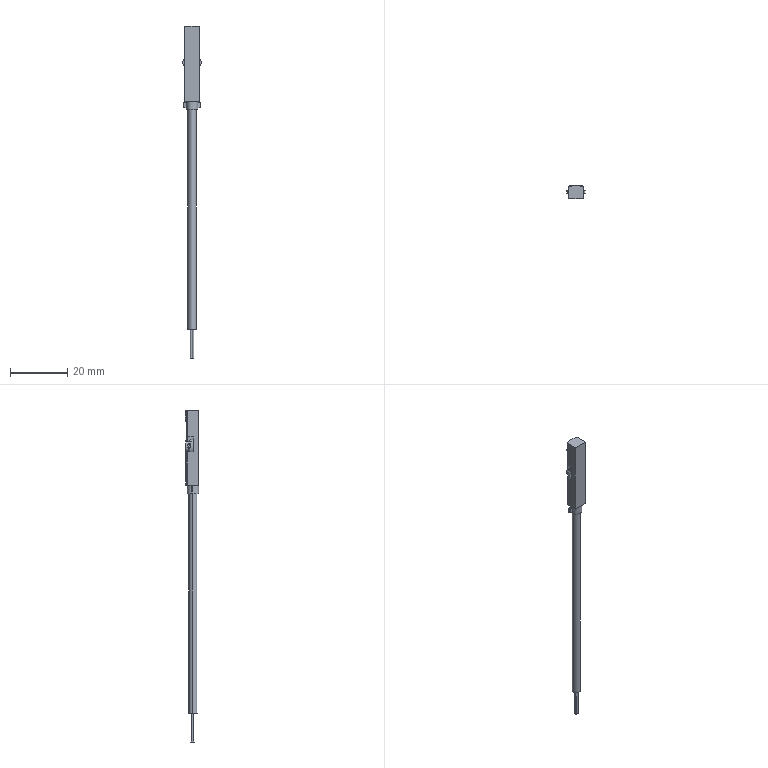Part | SolidWorks | features BaseBody 1 | 1 solid | 109 faces | box 6.45 x 4.8 x 116.3 mm | volume 1119 mm3 | plane 60 | cylinder 47 | cone 2 | commonest cylinder face diameters 0.4 x13 0.6 x6 0.2 x4 4 x4 4.6 x3 5.1 x3